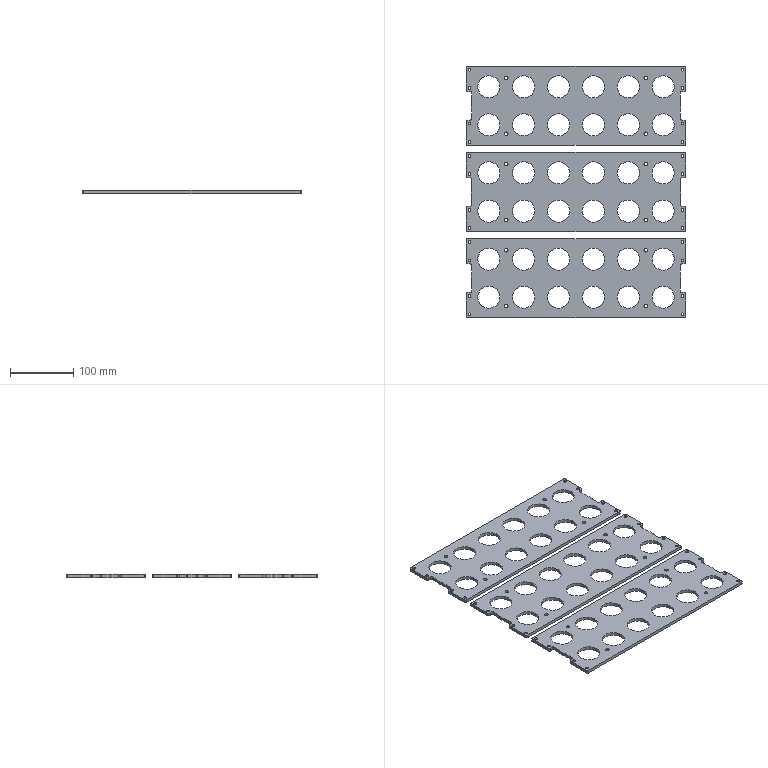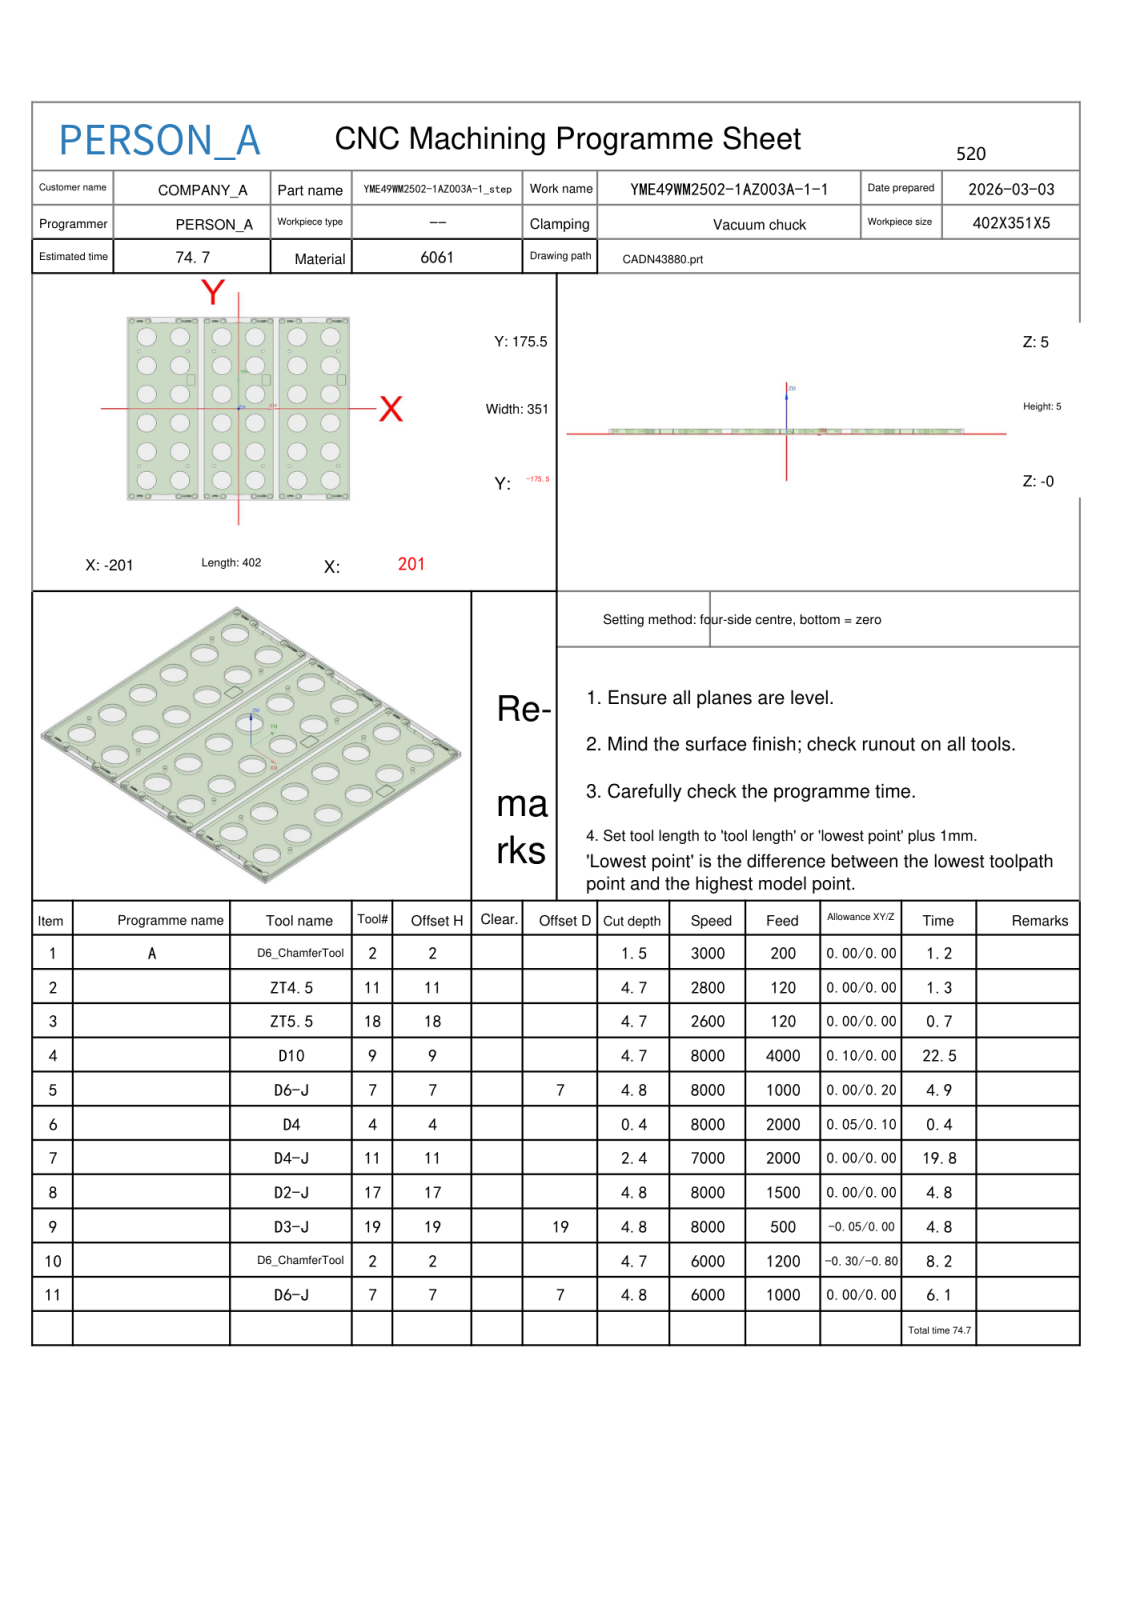NC program | NX | posted by the shop | part box 346 x 397 x 5 mm
Lines 1 to 161 of 51232:
%
O0001
(Machine time: 76.00 MIN)
(===Total Tool:8===)
(T2=D6_ChamferTool   D=6.   R=0.   D-  H02 Z=0.3   )
(T11=ZT4.5  D=4.5  DR_a=118 D-  H11 Z=0.3   )
(T18=ZT5.5  D=5.5  DR_a=118 D-  H18 Z=0.3   )
(T9=D10     D=10.  R=0.   D-  H09 Z=0.3   )
(T7=D6-J    D=6.   R=0.   D7  H07 Z=0.2   )
(T4=D4      D=4.   R=0.   D-  H04 Z=4.6   )
(T17=D2-J   D=2.   R=0.   D17 H17 Z=0.2   )
(T19=D3-J   D=3.   R=0.   D19 H19 Z=0.2   )
G80 G90 G17 G49 G40
G91 G28 Z0
M01
N1 T02 M06
(D6_ChamferTool  D=6. R=0. H=02 ce=0.00 di=0.00)
G00 G90 G54 X193. Y168. M03 S3000
G43 H02 Z35.
M08
G98 G81 X193. Y168. Z3.5 R6. F200.
X164.
X166. Y137.5
X180. Y110.
X166. Y82.5
Y27.5
Y-27.5
Y-82.5
X180. Y-110.
X166. Y-137.5
X193. Y-168.
X164.
X108.
X79.
X106. Y-137.5
X92. Y-110.
X106. Y-82.5
Y-27.5
Y27.5
Y82.5
X92. Y110.
X106. Y137.5
X108. Y168.
X79.
X57.
X28.
X30. Y137.5
X44. Y110.
X30. Y82.5
Y27.5
Y-27.5
Y-82.5
X44. Y-110.
X30. Y-137.5
X57. Y-168.
X28.
X-28.
X-57.
X-30. Y-137.5
X-44. Y-110.
X-30. Y-82.5
Y-27.5
Y27.5
Y82.5
X-44. Y110.
X-30. Y137.5
X-28. Y168.
X-57.
X-79.
X-108.
X-106. Y137.5
X-92. Y110.
X-106. Y82.5
Y27.5
Y-27.5
Y-82.5
X-92. Y-110.
X-106. Y-137.5
X-79. Y-168.
X-108.
X-164.
X-193.
X-166. Y-137.5
X-180. Y-110.
X-166. Y-82.5
Y-27.5
Y27.5
Y82.5
X-180. Y110.
X-166. Y137.5
X-164. Y168.
X-193.
G80
G00 Z35.
G91 G28 Z0.0
M05
M09
G91 G28 Z0.0
M01
N2 T11 M06
(ZT4.5 D=4.5 DR_a=118 H=11)
G00 G90 G54 X193. Y-168. M03 S2800
G43 H11 Z35.
M08
G98 G83 X193. Y-168. Z.3 R6. F120. Q1.5
X164.
X108.
X79.
X57.
X28.
X-28.
X-57.
X-79.
X-108.
X-164.
X-193.
Y168.
X-164.
X-108.
X-79.
X-57.
X-28.
X28.
X57.
X79.
X108.
X164.
X193.
G80
G00 Z35.
G91 G28 Z0.0
M05
M09
G91 G28 Z0.0
M01
N3 T18 M06
(ZT5.5 D=5.5 DR_a=118 H=18)
G00 G90 G54 X180. Y-110. M03 S2600
G43 H18 Z35.
M08
G98 G83 X180. Y-110. Z.3 R6. F120. Q1.5
X92.
X44.
X-44.
X-92.
X-180.
Y110.
X-92.
X-44.
X44.
X92.
X180.
G80
G00 Z35.
G91 G28 Z0.0
M05
M09
G91 G28 Z0.0
M01